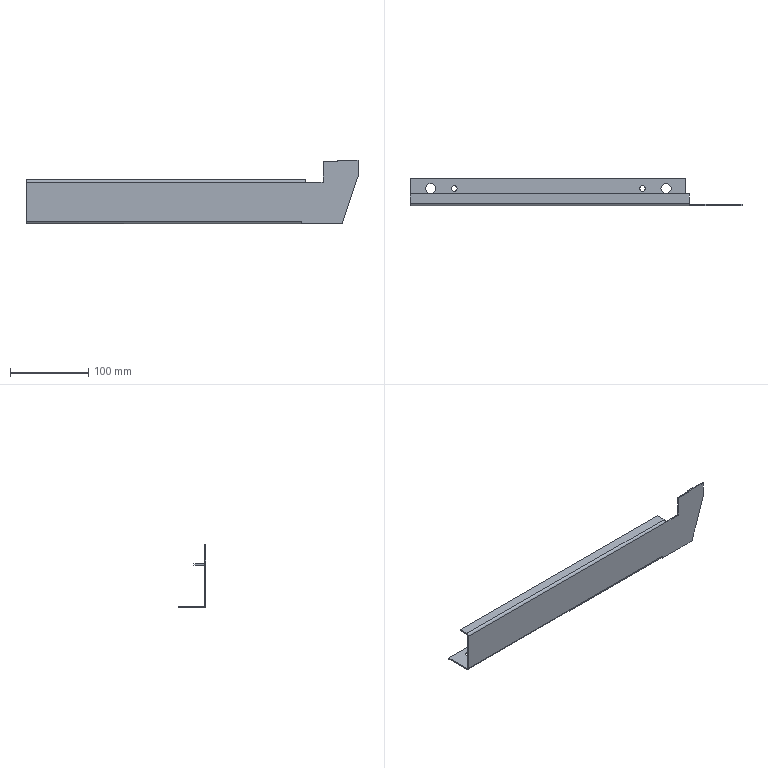Part | STEP file | Top flange baffle | 1 solid | 38 faces | box 423.333 x 35 x 81 mm | volume 59476 mm3 | plane 26 | cylinder 12 | commonest cylinder face diameters 7 x4 13 x4 3 x2 6 x2